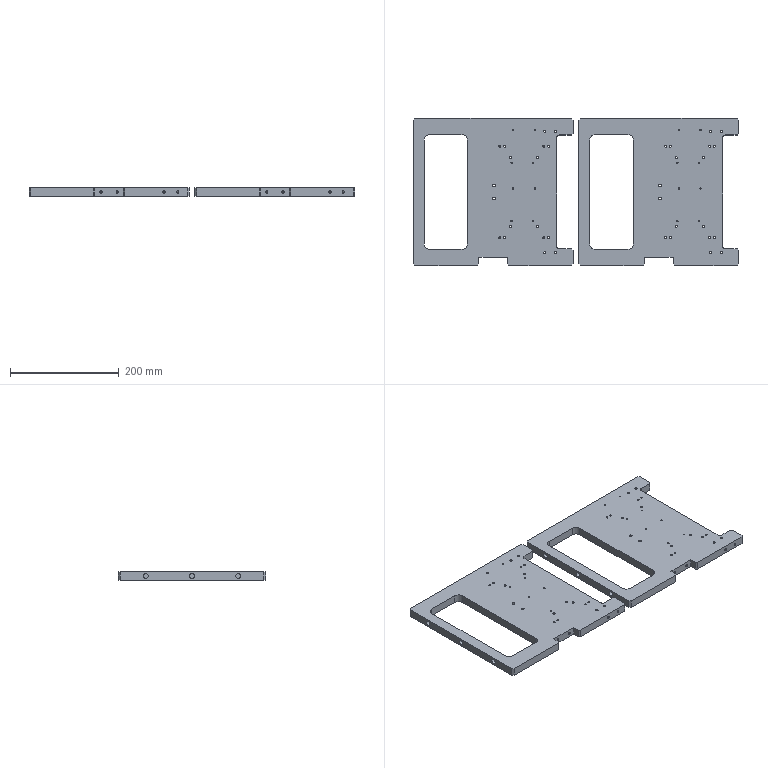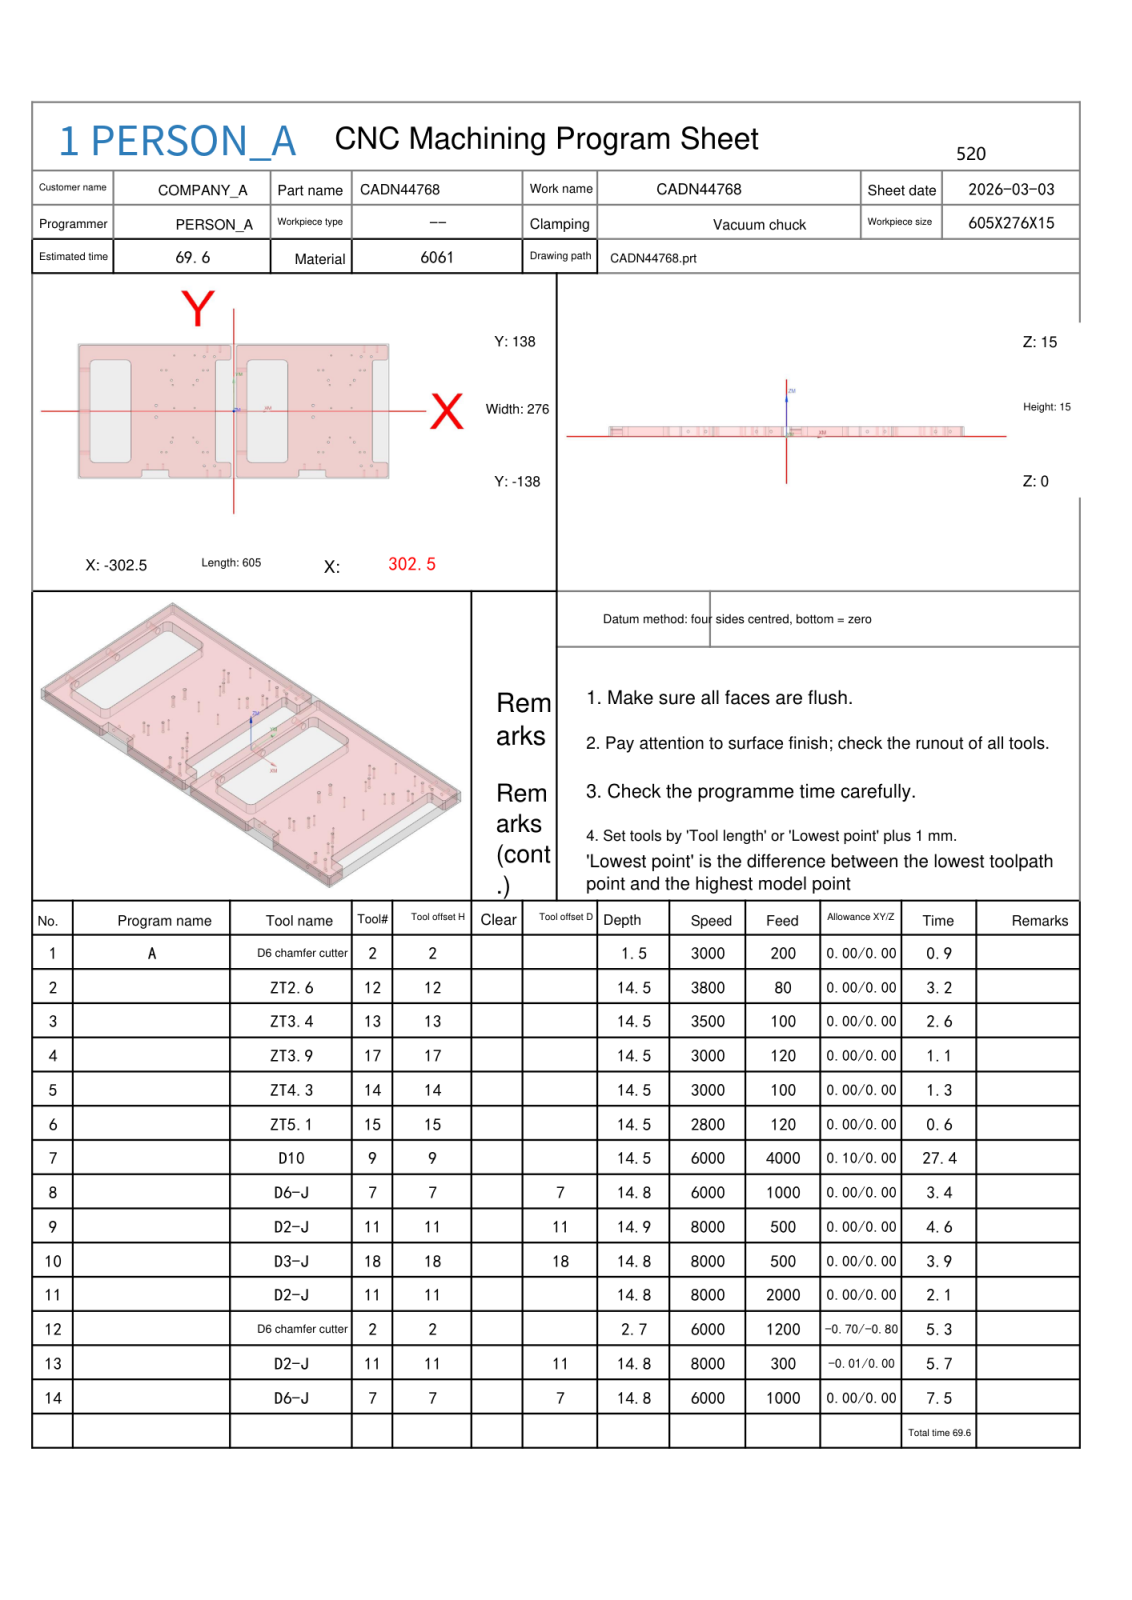NC program | NX | posted by the shop | part box 600 x 271 x 15 mm
Lines 1 to 205 of 17346:
%
O0001
(Machine time: 71.89 MIN)
(===Total Tool:10===)
(T2=D6 chamfer cutter   D=6.   R=0.   D-  H02 Z=12.3  )
(T12=ZT2.6  D=2.6  DR_a=118 D-  H12 Z=0.5   )
(T13=ZT3.4  D=3.4  DR_a=118 D-  H13 Z=0.5   )
(T17=ZT3.9  D=3.9  DR_a=120 D-  H17 Z=0.5   )
(T14=ZT4.3  D=4.3  DR_a=118 D-  H14 Z=0.5   )
(T15=ZT5.1  D=5.1  DR_a=118 D-  H15 Z=0.5   )
(T9=D10     D=10.  R=0.   D-  H09 Z=0.5   )
(T7=D6-J    D=6.   R=0.   D7  H07 Z=0.2   )
(T11=D2-J   D=2.   R=0.   D11 H11 Z=0.15  )
(T18=D3-J   D=3.   R=0.   D18 H18 Z=0.15  )
G80 G90 G17 G49 G40
G91 G28 Z0
M01
N1 T02 M06
(D6 chamfer cutter  D=6. R=0. H=02 ce=0.00 di=0.00)
(MAX_Z=45. MIN_Z=13.5 Time=0.80M)
G00 G90 G54 X186.75 Y-54. M03 S3000
G43 H02 Z45.
M08
G98 G81 X186.75 Y-54. Z14. R16. F200.
X226.75
X229.5 Y6.5
X189.5
X186.75 Y54.
X226.75
X229.5 Y114.5
X189.5
X-76.
X-116.
X-118.75 Y54.
X-78.75
X-76. Y6.5
X-116.
X-118.75 Y-54.
X-78.75
G80
G00 Z45.
G00 G90 X268. Y112. M03 S3000
Z45.
G98 G81 X268. Y112. Z13.5 R16. F200.
X248.
X255. Y84.
X246.
X234.5 Y63.5
X184.5
X174. Y84.
X165.
X154.5 Y12.
Y-12.
X184.5 Y-63.5
X234.5
X246. Y-84.
X255.
X268. Y-112.
X248.
X174. Y-84.
X165.
X-37.5 Y-112.
X-57.5
X-50.5 Y-84.
X-59.5
X-71. Y-63.5
X-121.
X-131.5 Y-84.
X-140.5
X-151. Y-12.
Y12.
X-140.5 Y84.
X-131.5
X-121. Y63.5
X-71.
X-59.5 Y84.
X-50.5
X-57.5 Y112.
X-37.5
G80
G00 Z45.
G91 G28 Z0.0
M05
M09
G91 G28 Z0.0
M01
N2 T12 M06
(ZT2.6 D=2.6 DR_a=118 H=12)
(MAX_Z=45. MIN_Z=0.5 Time=3.19M)
G00 G90 G54 X186.75 Y-54. M03 S3800
G43 H12 Z45.
M08
G98 G83 X186.75 Y-54. Z.5 R16. F80. Q1.5
X226.75
X229.5 Y6.5
X189.5
X186.75 Y54.
X226.75
X229.5 Y114.5
X189.5
X-76.
X-116.
X-118.75 Y54.
X-78.75
X-76. Y6.5
X-116.
X-118.75 Y-54.
X-78.75
G80
G00 Z45.
G91 G28 Z0.0
M05
M09
G91 G28 Z0.0
M01
N3 T13 M06
(ZT3.4 D=3.4 DR_a=118 H=13)
(MAX_Z=45. MIN_Z=0.5 Time=2.55M)
G00 G90 G54 X-50.5 Y-84. M03 S3500
G43 H13 Z45.
M08
G98 G83 X-50.5 Y-84. Z.5 R16. F100. Q1.5
X-59.5
X-131.5
X-140.5
Y84.
X-131.5
X-59.5
X-50.5
X165.
X174.
X246.
X255.
Y-84.
X246.
X174.
X165.
G80
G00 Z45.
G91 G28 Z0.0
M05
M09
G91 G28 Z0.0
M01
N4 T17 M06
(ZT3.9 D=3.9 DR_a=120 H=17)
(MAX_Z=45. MIN_Z=0.5 Time=1.10M)
G00 G90 G54 X-71. Y-63.5 M03 S3000
G43 H17 Z45.
M08
G98 G83 X-71. Y-63.5 Z.5 R16. F120. Q2.
X-121.
Y63.5
X-71.
X184.5
X234.5
Y-63.5
X184.5
G80
G00 Z45.
G91 G28 Z0.0
M05
M09
G91 G28 Z0.0
M01
N5 T14 M06
(ZT4.3 D=4.3 DR_a=118 H=14)
(MAX_Z=45. MIN_Z=0.5 Time=1.31M)
G00 G90 G54 X-37.5 Y-112. M03 S3000
G43 H14 Z45.
M08
G98 G83 X-37.5 Y-112. Z.5 R16. F100. Q1.5
X-57.5
Y112.
X-37.5
X248.
X268.
Y-112.
X248.
G80
G00 Z45.
G91 G28 Z0.0
M05
M09
G91 G28 Z0.0
M01
N6 T15 M06
(ZT5.1 D=5.1 DR_a=118 H=15)
(MAX_Z=45. MIN_Z=0.5 Time=0.55M)
G00 G90 G54 X154.5 Y-12. M03 S2800
G43 H15 Z45.
M08
G98 G83 X154.5 Y-12. Z.5 R16. F120. Q1.5
Y12.
X-151.
Y-12.
G80
G00 Z45.
G91 G28 Z0.0
M05
M09
G91 G28 Z0.0
M01